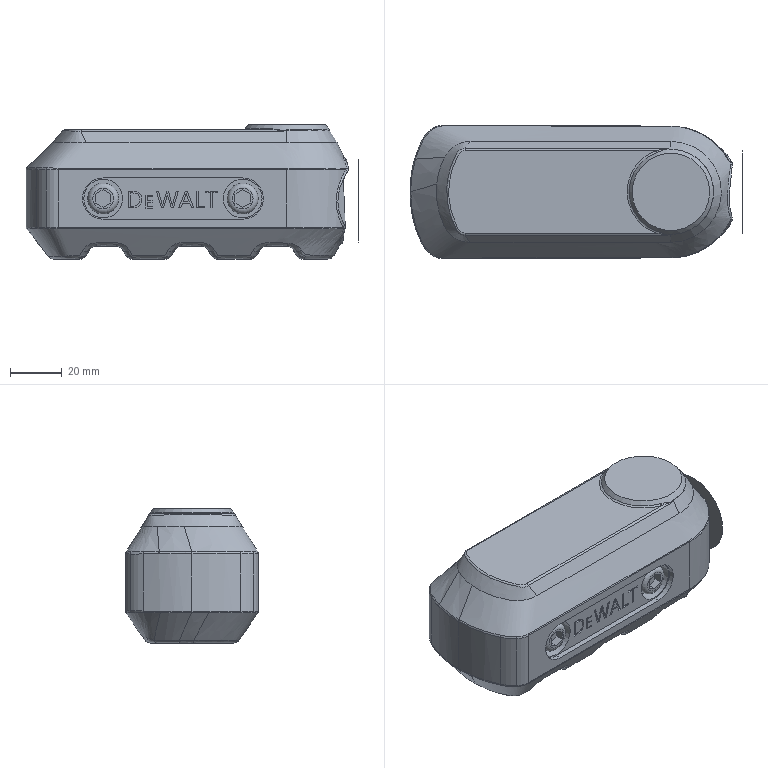Part | STEP file | DEWALT-DWE7492-B22 | 1 solid | 332 faces | box 128.5 x 51.395 x 52 mm | volume 252814 mm3 | plane 174 | spline 103 | cylinder 34 | sphere 12 | torus 6 | cone 3 | commonest cylinder face diameters 6 x12 12 x4 15 x4 16 x4 2 x2 13.922 x2